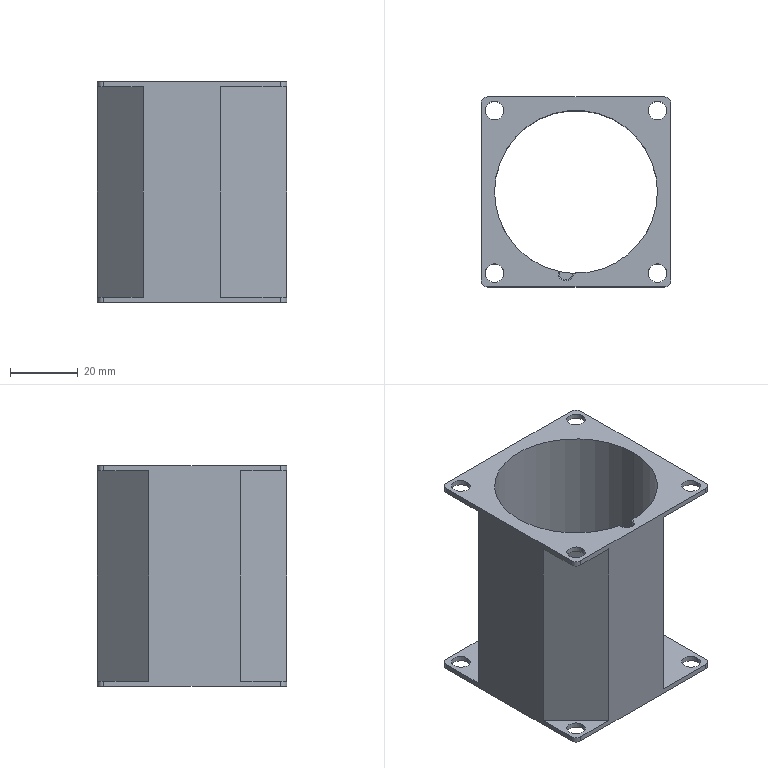Part | STEP file | 连接Plate 2 | 1 solid | 51 faces | box 56 x 56 x 65.079 mm | volume 55529 mm3 | cylinder 29 | plane 19 | cone 3 | commonest cylinder face diameters 5.5 x16 4 x11 48 x2